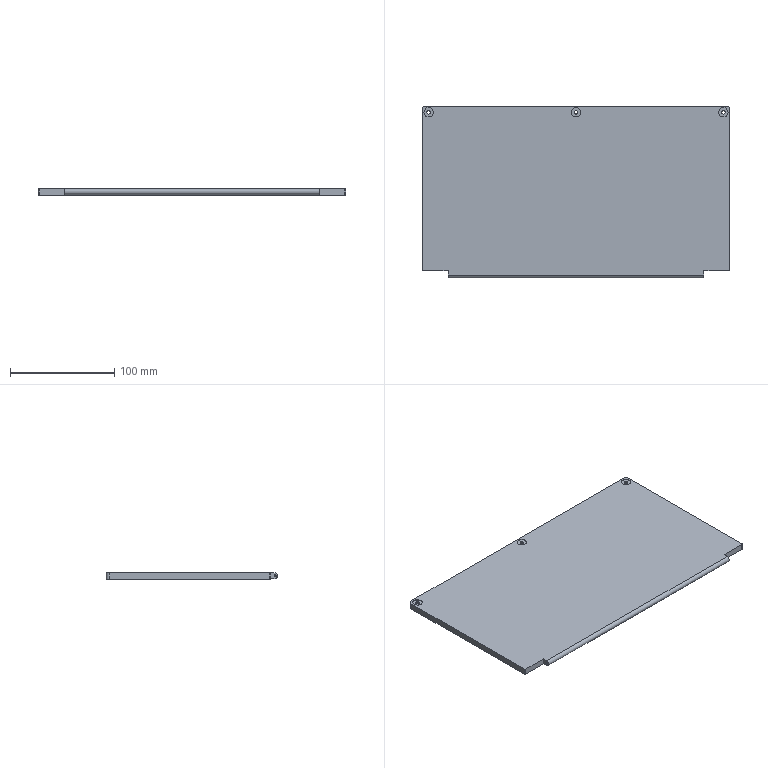NC program | Mastercam | posted with a generic post
Lines 1 to 867 of 5159:
%
O0000()
(MATERIAL - ALUMINUM MM - 2024)
( T9 | 10 FEM | H9 | XY STOCK TO LEAVE - 5. | Z STOCK TO LEAVE - .05 )
( T10 | 10 FEM | H10 | XY STOCK TO LEAVE - 0. | Z STOCK TO LEAVE - .05 )
( T1 | 4 BNOS | H1 )
( T6 | 6 FEM | H6 | XY STOCK TO LEAVE - -.01 | Z STOCK TO LEAVE - 0. )
( T5 | 4 CHM | H5 )
( T3 | 3 FEM | H3 | XY STOCK TO LEAVE - -.01 | Z STOCK TO LEAVE - 0. )
( T8 | 8 FEM | H8 | XY STOCK TO LEAVE - .1 | Z STOCK TO LEAVE - .1 )
N100 G21
N110 G0 G17 G40 G49 G80 G90
N120 T9 M6
N130 G0 G90 G54 X-132.7 Y-102.5 A0. S7000 M3
N140 G43 H9 Z50. M8
N150 Z1.
N160 G1 Z-.496 F600.
N170 Y-92.5 F3000.
N180 Y-85.5
N190 X-146.5
N200 X-156.5
N210 Z-.992 F600.
N220 X-146.5 F3000.
N230 X-132.7
N240 Y-92.5
N250 Y-102.5
N260 Z-1.488 F600.
N270 Y-92.5 F3000.
N280 Y-85.5
N290 X-146.5
N300 X-156.5
N310 Z-1.983 F600.
N320 X-146.5 F3000.
N330 X-132.7
N340 Y-92.5
N350 Y-102.5
N360 Z-2.479 F600.
N370 Y-92.5 F3000.
N380 Y-85.5
N390 X-146.5
N400 X-156.5
N410 Z-2.975 F600.
N420 X-146.5 F3000.
N430 X-132.7
N440 Y-92.5
N450 Y-102.5
N460 Z-3.471 F600.
N470 Y-92.5 F3000.
N480 Y-85.5
N490 X-146.5
N500 X-156.5
N510 Z-3.967 F600.
N520 X-146.5 F3000.
N530 X-132.7
N540 Y-92.5
N550 Y-102.5
N560 Z-4.463 F600.
N570 Y-92.5 F3000.
N580 Y-85.5
N590 X-146.5
N600 X-156.5
N610 Z-4.958 F600.
N620 X-146.5 F3000.
N630 X-132.7
N640 Y-92.5
N650 Y-102.5
N660 Z-5.454 F600.
N670 Y-92.5 F3000.
N680 Y-85.5
N690 X-146.5
N700 X-156.5
N710 Z-5.95 F600.
N720 X-146.5 F3000.
N730 X-132.7
N740 Y-92.5
N750 Y-102.5
N760 G0 Z50.
N770 X156.5 Y-85.5
N780 Z1.
N790 G1 Z-.496 F600.
N800 X146.5 F3000.
N810 X132.7
N820 Y-92.5
N830 Y-102.5
N840 Z-.992 F600.
N850 Y-92.5 F3000.
N860 Y-85.5
N870 X146.5
N880 X156.5
N890 Z-1.488 F600.
N900 X146.5 F3000.
N910 X132.7
N920 Y-92.5
N930 Y-102.5
N940 Z-1.983 F600.
N950 Y-92.5 F3000.
N960 Y-85.5
N970 X146.5
N980 X156.5
N990 Z-2.479 F600.
N1000 X146.5 F3000.
N1010 X132.7
N1020 Y-92.5
N1030 Y-102.5
N1040 Z-2.975 F600.
N1050 Y-92.5 F3000.
N1060 Y-85.5
N1070 X146.5
N1080 X156.5
N1090 Z-3.471 F600.
N1100 X146.5 F3000.
N1110 X132.7
N1120 Y-92.5
N1130 Y-102.5
N1140 Z-3.967 F600.
N1150 Y-92.5 F3000.
N1160 Y-85.5
N1170 X146.5
N1180 X156.5
N1190 Z-4.463 F600.
N1200 X146.5 F3000.
N1210 X132.7
N1220 Y-92.5
N1230 Y-102.5
N1240 Z-4.958 F600.
N1250 Y-92.5 F3000.
N1260 Y-85.5
N1270 X146.5
N1280 X156.5
N1290 Z-5.454 F600.
N1300 X146.5 F3000.
N1310 X132.7
N1320 Y-92.5
N1330 Y-102.5
N1340 Z-5.95 F600.
N1350 Y-92.5 F3000.
N1360 Y-85.5
N1370 X146.5
N1380 X156.5
N1390 G0 Z50.
N1400 X-145.5 Y89.65
N1410 Z1.
N1420 G1 Z0. F600.
N1430 Y88.65 F3000.
N1440 G3 X-144.5 Y87.65 I1. J0.
N1450 G1 X144.5 Z-.153
N1460 G2 X152.65 Y79.5 Z-.16 I0. J-8.15
N1470 G1 Y-74.5 Z-.241
N1480 G2 X146.5 Y-80.65 Z-.246 I-6.15 J0.
N1490 G1 X128.2 Z-.256
N1500 G3 X127.85 Y-81. I0. J-.35
N1510 G1 Y-82.5 Z-.257
N1520 G2 X122.7 Y-87.65 Z-.262 I-5.15 J0.
N1530 G1 X-122.7 Z-.391
N1540 G2 X-127.85 Y-82.5 Z-.396 I0. J5.15
N1550 G1 Y-81. Z-.397
N1560 G3 X-128.2 Y-80.65 I-.35 J0.
N1570 G1 X-146.5 Z-.407
N1580 G2 X-152.65 Y-74.5 Z-.412 I0. J6.15
N1590 G1 Y79.5 Z-.493
N1600 G2 X-144.5 Y87.65 Z-.5 I8.15 J0.
N1610 G1 X144.5 Z-.653
N1620 G2 X152.65 Y79.5 Z-.66 I0. J-8.15
N1630 G1 Y-74.5 Z-.741
N1640 G2 X146.5 Y-80.65 Z-.746 I-6.15 J0.
N1650 G1 X128.2 Z-.756
N1660 G3 X127.85 Y-81. I0. J-.35
N1670 G1 Y-82.5 Z-.757
N1680 G2 X122.7 Y-87.65 Z-.762 I-5.15 J0.
N1690 G1 X-122.7 Z-.891
N1700 G2 X-127.85 Y-82.5 Z-.896 I0. J5.15
N1710 G1 Y-81. Z-.897
N1720 G3 X-128.2 Y-80.65 I-.35 J0.
N1730 G1 X-146.5 Z-.907
N1740 G2 X-152.65 Y-74.5 Z-.912 I0. J6.15
N1750 G1 Y79.5 Z-.993
N1760 G2 X-144.5 Y87.65 Z-1. I8.15 J0.
N1770 G1 X144.5 Z-1.153
N1780 G2 X152.65 Y79.5 Z-1.16 I0. J-8.15
N1790 G1 Y-74.5 Z-1.241
N1800 G2 X146.5 Y-80.65 Z-1.246 I-6.15 J0.
N1810 G1 X128.2 Z-1.256
N1820 G3 X127.85 Y-81. I0. J-.35
N1830 G1 Y-82.5 Z-1.257
N1840 G2 X122.7 Y-87.65 Z-1.262 I-5.15 J0.
N1850 G1 X-122.7 Z-1.391
N1860 G2 X-127.85 Y-82.5 Z-1.396 I0. J5.15
N1870 G1 Y-81. Z-1.397
N1880 G3 X-128.2 Y-80.65 I-.35 J0.
N1890 G1 X-146.5 Z-1.407
N1900 G2 X-152.65 Y-74.5 Z-1.412 I0. J6.15
N1910 G1 Y79.5 Z-1.493
N1920 G2 X-144.5 Y87.65 Z-1.5 I8.15 J0.
N1930 G1 X144.5 Z-1.653
N1940 G2 X152.65 Y79.5 Z-1.66 I0. J-8.15
N1950 G1 Y-74.5 Z-1.741
N1960 G2 X146.5 Y-80.65 Z-1.746 I-6.15 J0.
N1970 G1 X128.2 Z-1.756
N1980 G3 X127.85 Y-81. I0. J-.35
N1990 G1 Y-82.5 Z-1.757
N2000 G2 X122.7 Y-87.65 Z-1.762 I-5.15 J0.
N2010 G1 X-122.7 Z-1.891
N2020 G2 X-127.85 Y-82.5 Z-1.896 I0. J5.15
N2030 G1 Y-81. Z-1.897
N2040 G3 X-128.2 Y-80.65 I-.35 J0.
N2050 G1 X-146.5 Z-1.907
N2060 G2 X-152.65 Y-74.5 Z-1.912 I0. J6.15
N2070 G1 Y79.5 Z-1.993
N2080 G2 X-144.5 Y87.65 Z-2. I8.15 J0.
N2090 G1 X144.5 Z-2.153
N2100 G2 X152.65 Y79.5 Z-2.16 I0. J-8.15
N2110 G1 Y-74.5 Z-2.241
N2120 G2 X146.5 Y-80.65 Z-2.246 I-6.15 J0.
N2130 G1 X128.2 Z-2.256
N2140 G3 X127.85 Y-81. I0. J-.35
N2150 G1 Y-82.5 Z-2.257
N2160 G2 X122.7 Y-87.65 Z-2.262 I-5.15 J0.
N2170 G1 X-122.7 Z-2.391
N2180 G2 X-127.85 Y-82.5 Z-2.396 I0. J5.15
N2190 G1 Y-81. Z-2.397
N2200 G3 X-128.2 Y-80.65 I-.35 J0.
N2210 G1 X-146.5 Z-2.407
N2220 G2 X-152.65 Y-74.5 Z-2.412 I0. J6.15
N2230 G1 Y79.5 Z-2.493
N2240 G2 X-144.5 Y87.65 Z-2.5 I8.15 J0.
N2250 G1 X144.5 Z-2.653
N2260 G2 X152.65 Y79.5 Z-2.66 I0. J-8.15
N2270 G1 Y-74.5 Z-2.741
N2280 G2 X146.5 Y-80.65 Z-2.746 I-6.15 J0.
N2290 G1 X128.2 Z-2.756
N2300 G3 X127.85 Y-81. I0. J-.35
N2310 G1 Y-82.5 Z-2.757
N2320 G2 X122.7 Y-87.65 Z-2.762 I-5.15 J0.
N2330 G1 X-122.7 Z-2.891
N2340 G2 X-127.85 Y-82.5 Z-2.896 I0. J5.15
N2350 G1 Y-81. Z-2.897
N2360 G3 X-128.2 Y-80.65 I-.35 J0.
N2370 G1 X-146.5 Z-2.907
N2380 G2 X-152.65 Y-74.5 Z-2.912 I0. J6.15
N2390 G1 Y79.5 Z-2.993
N2400 G2 X-144.5 Y87.65 Z-3. I8.15 J0.
N2410 G1 X144.5 Z-3.153
N2420 G2 X152.65 Y79.5 Z-3.16 I0. J-8.15
N2430 G1 Y-74.5 Z-3.241
N2440 G2 X146.5 Y-80.65 Z-3.246 I-6.15 J0.
N2450 G1 X128.2 Z-3.256
N2460 G3 X127.85 Y-81. I0. J-.35
N2470 G1 Y-82.5 Z-3.257
N2480 G2 X122.7 Y-87.65 Z-3.262 I-5.15 J0.
N2490 G1 X-122.7 Z-3.391
N2500 G2 X-127.85 Y-82.5 Z-3.396 I0. J5.15
N2510 G1 Y-81. Z-3.397
N2520 G3 X-128.2 Y-80.65 I-.35 J0.
N2530 G1 X-146.5 Z-3.407
N2540 G2 X-152.65 Y-74.5 Z-3.412 I0. J6.15
N2550 G1 Y79.5 Z-3.493
N2560 G2 X-144.5 Y87.65 Z-3.5 I8.15 J0.
N2570 G1 X144.5 Z-3.653
N2580 G2 X152.65 Y79.5 Z-3.66 I0. J-8.15
N2590 G1 Y-74.5 Z-3.741
N2600 G2 X146.5 Y-80.65 Z-3.746 I-6.15 J0.
N2610 G1 X128.2 Z-3.756
N2620 G3 X127.85 Y-81. I0. J-.35
N2630 G1 Y-82.5 Z-3.757
N2640 G2 X122.7 Y-87.65 Z-3.762 I-5.15 J0.
N2650 G1 X-122.7 Z-3.891
N2660 G2 X-127.85 Y-82.5 Z-3.896 I0. J5.15
N2670 G1 Y-81. Z-3.897
N2680 G3 X-128.2 Y-80.65 I-.35 J0.
N2690 G1 X-146.5 Z-3.907
N2700 G2 X-152.65 Y-74.5 Z-3.912 I0. J6.15
N2710 G1 Y79.5 Z-3.993
N2720 G2 X-144.5 Y87.65 Z-4. I8.15 J0.
N2730 G1 X144.5 Z-4.153
N2740 G2 X152.65 Y79.5 Z-4.16 I0. J-8.15
N2750 G1 Y-74.5 Z-4.241
N2760 G2 X146.5 Y-80.65 Z-4.246 I-6.15 J0.
N2770 G1 X128.2 Z-4.256
N2780 G3 X127.85 Y-81. I0. J-.35
N2790 G1 Y-82.5 Z-4.257
N2800 G2 X122.7 Y-87.65 Z-4.262 I-5.15 J0.
N2810 G1 X-122.7 Z-4.391
N2820 G2 X-127.85 Y-82.5 Z-4.396 I0. J5.15
N2830 G1 Y-81. Z-4.397
N2840 G3 X-128.2 Y-80.65 I-.35 J0.
N2850 G1 X-146.5 Z-4.407
N2860 G2 X-152.65 Y-74.5 Z-4.412 I0. J6.15
N2870 G1 Y79.5 Z-4.493
N2880 G2 X-144.5 Y87.65 Z-4.5 I8.15 J0.
N2890 G1 X144.5 Z-4.653
N2900 G2 X152.65 Y79.5 Z-4.66 I0. J-8.15
N2910 G1 Y-74.5 Z-4.741
N2920 G2 X146.5 Y-80.65 Z-4.746 I-6.15 J0.
N2930 G1 X128.2 Z-4.756
N2940 G3 X127.85 Y-81. I0. J-.35
N2950 G1 Y-82.5 Z-4.757
N2960 G2 X122.7 Y-87.65 Z-4.762 I-5.15 J0.
N2970 G1 X-122.7 Z-4.891
N2980 G2 X-127.85 Y-82.5 Z-4.896 I0. J5.15
N2990 G1 Y-81. Z-4.897
N3000 G3 X-128.2 Y-80.65 I-.35 J0.
N3010 G1 X-146.5 Z-4.907
N3020 G2 X-152.65 Y-74.5 Z-4.912 I0. J6.15
N3030 G1 Y79.5 Z-4.993
N3040 G2 X-144.5 Y87.65 Z-5. I8.15 J0.
N3050 G1 X144.5 Z-5.153
N3060 G2 X152.65 Y79.5 Z-5.16 I0. J-8.15
N3070 G1 Y-74.5 Z-5.241
N3080 G2 X146.5 Y-80.65 Z-5.246 I-6.15 J0.
N3090 G1 X128.2 Z-5.256
N3100 G3 X127.85 Y-81. I0. J-.35
N3110 G1 Y-82.5 Z-5.257
N3120 G2 X122.7 Y-87.65 Z-5.262 I-5.15 J0.
N3130 G1 X-122.7 Z-5.391
N3140 G2 X-127.85 Y-82.5 Z-5.396 I0. J5.15
N3150 G1 Y-81. Z-5.397
N3160 G3 X-128.2 Y-80.65 I-.35 J0.
N3170 G1 X-146.5 Z-5.407
N3180 G2 X-152.65 Y-74.5 Z-5.412 I0. J6.15
N3190 G1 Y79.5 Z-5.493
N3200 G2 X-144.5 Y87.65 Z-5.5 I8.15 J0.
N3210 G1 X144.5 Z-5.653
N3220 G2 X152.65 Y79.5 Z-5.66 I0. J-8.15
N3230 G1 Y-74.5 Z-5.741
N3240 G2 X146.5 Y-80.65 Z-5.746 I-6.15 J0.
N3250 G1 X128.2 Z-5.756
N3260 G3 X127.85 Y-81. I0. J-.35
N3270 G1 Y-82.5 Z-5.757
N3280 G2 X122.7 Y-87.65 Z-5.762 I-5.15 J0.
N3290 G1 X-122.7 Z-5.891
N3300 G2 X-127.85 Y-82.5 Z-5.896 I0. J5.15
N3310 G1 Y-81. Z-5.897
N3320 G3 X-128.2 Y-80.65 I-.35 J0.
N3330 G1 X-146.5 Z-5.907
N3340 G2 X-152.65 Y-74.5 Z-5.912 I0. J6.15
N3350 G1 Y-2.118 Z-5.95
N3360 Y79.5
N3370 G2 X-144.5 Y87.65 I8.15 J0.
N3380 G1 X144.5
N3390 G2 X152.65 Y79.5 I0. J-8.15
N3400 G1 Y-74.5
N3410 G2 X146.5 Y-80.65 I-6.15 J0.
N3420 G1 X128.2
N3430 G3 X127.85 Y-81. I0. J-.35
N3440 G1 Y-82.5
N3450 G2 X122.7 Y-87.65 I-5.15 J0.
N3460 G1 X-122.7
N3470 G2 X-127.85 Y-82.5 I0. J5.15
N3480 G1 Y-81.
N3490 G3 X-128.2 Y-80.65 I-.35 J0.
N3500 G1 X-146.5
N3510 G2 X-152.65 Y-74.5 I0. J6.15
N3520 G1 Y-2.118
N3530 G3 X-153.65 Y-1.118 I-1. J0.
N3540 G1 X-154.65
N3550 G0 Z50.
N3560 M5
N3570 G91 G28 Z0. M9
N3580 A0.
N3590 M01
N3600 T10 M6
N3610 G0 G90 G17 G54 X-145.5 Y89.5 A0. S7000 M3
N3620 G43 H10 Z50. M8
N3630 Z1.
N3640 G1 Z-5.95 F600.
N3650 Y88.5 F1000.
N3660 G3 X-144.5 Y87.5 I1. J0.
N3670 G1 X144.5
N3680 G2 X152.5 Y79.5 I0. J-8.
N3690 G1 Y-74.5
N3700 G2 X146.5 Y-80.5 I-6. J0.
N3710 G1 X128.2
N3720 G3 X127.7 Y-81. I0. J-.5
N3730 G1 Y-82.5
N3740 G2 X122.7 Y-87.5 I-5. J0.
N3750 G1 X-122.7
N3760 G2 X-127.7 Y-82.5 I0. J5.
N3770 G1 Y-81.
N3780 G3 X-128.2 Y-80.5 I-.5 J0.
N3790 G1 X-146.5
N3800 G2 X-152.5 Y-74.5 I0. J6.
N3810 G1 Y79.5
N3820 G2 X-144.5 Y87.5 I8. J0.
N3830 G3 X-143.5 Y88.5 I0. J1.
N3840 G1 Y89.5
N3850 G0 Z50.
N3860 M5
N3870 G91 G28 Z0. M9
N3880 A0.
N3890 M01
N3900 T1 M6
N3910 G0 G90 G17 G54 X132.7 Y-84.49 A0. S10000 M3
N3920 G43 H1 Z50. M8
N3930 Z.929
N3940 G1 Z-3.693 F600.
N3950 X122.7 F3000.
N3960 Z-4.071 F600.
N3970 X-122.7 F3000.
N3980 Z-3.693
N3990 X-132.7
N4000 Z-3.936
N4010 Y-84.498
N4020 X-122.7
N4030 X122.7
N4040 X132.7
N4050 Z-3.8
N4060 Y-84.5
N4070 X122.7
N4080 X-122.7
N4090 X-132.7
N4100 Z-3.664
N4110 Y-84.498
N4120 X-122.7
N4130 X122.7
N4140 X132.7
N4150 Z-3.529
N4160 Y-84.49
N4170 X122.7
N4180 X-122.7
N4190 X-132.7
N4200 Z-3.394
N4210 Y-84.478
N4220 X-122.7
N4230 X122.7
N4240 X132.7
N4250 Z-3.26
N4260 Y-84.461
N4270 X122.7
N4280 X-122.7
N4290 X-132.7
N4300 Z-3.127
N4310 Y-84.44
N4320 X-122.7
N4330 X122.7
N4340 X132.7
N4350 Z-2.996
N4360 Y-84.414
N4370 X122.7
N4380 X-122.7
N4390 X-132.7
N4400 Z-2.865
N4410 Y-84.383
N4420 X-122.7
N4430 X122.7
N4440 X132.7
N4450 Z-2.737
N4460 Y-84.348
N4470 X122.7
N4480 X-122.7
N4490 X-132.7
N4500 Z-2.61
N4510 Y-84.309
N4520 X-122.7
N4530 X122.7
N4540 X132.7
N4550 Z-2.486
N4560 Y-84.265
N4570 X122.7
N4580 X-122.7
N4590 X-132.7
N4600 Z-2.364
N4610 Y-84.218
N4620 X-122.7
N4630 X122.7
N4640 X132.7
N4650 Z-2.244
N4660 Y-84.167
N4670 X122.7
N4680 X-122.7
N4690 X-132.7
N4700 Z-2.127
N4710 Y-84.112
N4720 X-122.7
N4730 X122.7
N4740 X132.7
N4750 Z-2.013
N4760 Y-84.054
N4770 X122.7
N4780 X-122.7
N4790 X-132.7
N4800 Z-1.902
N4810 Y-83.992
N4820 X-122.7
N4830 X122.7
N4840 X132.7
N4850 Z-1.794
N4860 Y-83.927
N4870 X122.7
N4880 X-122.7
N4890 X-132.7
N4900 Z-1.689
N4910 Y-83.86
N4920 X-122.7
N4930 X122.7
N4940 X132.7
N4950 Z-1.587
N4960 Y-83.789
N4970 X122.7
N4980 X-122.7
N4990 X-132.7
N5000 Z-1.489
N5010 Y-83.716
N5020 X-122.7
N5030 X122.7
N5040 X132.7
N5050 Z-1.394
N5060 Y-83.641
N5070 X122.7
N5080 X-122.7
N5090 X-132.7
N5100 Z-1.303
N5110 Y-83.564
N5120 X-122.7
N5130 X122.7
N5140 X132.7
N5150 Z-1.215
N5160 Y-83.485
N5170 X122.7
N5180 X-122.7
N5190 X-132.7
N5200 Z-1.13
N5210 Y-83.404
N5220 X-122.7
N5230 X122.7
N5240 X132.7
N5250 Z-1.05
N5260 Y-83.322
N5270 X122.7
N5280 X-122.7
N5290 X-132.7
N5300 Z-.972
N5310 Y-83.239
N5320 X-122.7
N5330 X122.7
N5340 X132.7
N5350 Z-.899
N5360 Y-83.154
N5370 X122.7
N5380 X-122.7
N5390 X-132.7
N5400 Z-.828
N5410 Y-83.068
N5420 X-122.7
N5430 X122.7
N5440 X132.7
N5450 Z-.761
N5460 Y-82.982
N5470 X122.7
N5480 X-122.7
N5490 X-132.7
N5500 Z-.681
N5510 Y-82.871
N5520 X-122.7
N5530 X122.7
N5540 X132.7
N5550 Z-.606
N5560 Y-82.759
N5570 X122.7
N5580 X-122.7
N5590 X-132.7
N5600 Z-.537
N5610 Y-82.647
N5620 X-122.7
N5630 X122.7
N5640 X132.7
N5650 Z-.472
N5660 Y-82.535
N5670 X122.7
N5680 X-122.7
N5690 X-132.7
N5700 Z-.413
N5710 Y-82.423
N5720 X-122.7
N5730 X122.7
N5740 X132.7
N5750 Z-.358
N5760 Y-82.311
N5770 X122.7
N5780 X-122.7
N5790 X-132.7
N5800 Z-.309
N5810 Y-82.2
N5820 X-122.7
N5830 X122.7
N5840 X132.7
N5850 Z-.263
N5860 Y-82.09
N5870 X122.7
N5880 X-122.7
N5890 X-132.7
N5900 Z-.222
N5910 Y-81.98
N5920 X-122.7
N5930 X122.7
N5940 X132.7
N5950 Z-.185
N5960 Y-81.872
N5970 X122.7
N5980 X-122.7
N5990 X-132.7
N6000 Z-.152
N6010 Y-81.765
N6020 X-122.7
N6030 X122.7
N6040 X132.7
N6050 Z-.123
N6060 Y-81.66
N6070 X122.7
N6080 X-122.7
N6090 X-132.7
N6100 Z-.098
N6110 Y-81.556
N6120 X-122.7
N6130 X122.7
N6140 X132.7
N6150 Z-.075
N6160 Y-81.453
N6170 X122.7
N6180 X-122.7
N6190 X-132.7
N6200 Z-.056
N6210 Y-81.353
N6220 X-122.7
N6230 X122.7
N6240 X132.7
N6250 Z-.041
N6260 Y-81.254
N6270 X122.7
N6280 X-122.7
N6290 X-132.7
N6300 Z-.028
N6310 Y-81.157
N6320 X-122.7
N6330 X122.7
N6340 X132.7
N6350 Z-.017
N6360 Y-81.061
N6370 X122.7
N6380 X-122.7
N6390 X-132.7
N6400 Z-.009
N6410 Y-80.968
N6420 X-122.7
N6430 X122.7
N6440 X132.7
N6450 Z-.004
N6460 Y-80.877
N6470 X122.7
N6480 X-122.7
N6490 X-132.7
N6500 Z-.001
N6510 Y-80.787
N6520 X-122.7
N6530 X122.7
N6540 X132.7
N6550 Z0.
N6560 Y-80.7
N6570 X122.7
N6580 X-122.7
N6590 X-132.7
N6600 G0 Z5.
N6610 Z50.
N6620 M5
N6630 G91 G28 Z0. M9
N6640 A0.
N6650 M01
N6660 T6 M6
N6670 G0 G90 G17 G54 X0. Y76.5 A0. S7000 M3
N6680 G43 H6 Z50. M8
N6690 Z1.
N6700 G1 Z0. F600.
N6710 X-.329 Y75.559 F3000.
N6720 G3 X.306 Y75.16 I.635 J.306
N6730 X.612 Y75.23 I0. J.705
N6740 X1.41 Y76.5 Z-.062 I-.612 J1.27
N6750 X0. Y77.91 Z-.15 I-1.41 J0.
N6760 X-1.41 Y76.5 Z-.237 I0. J-1.41
N6770 X0. Y75.09 Z-.325 I1.41 J0.
N6780 X.612 Y75.23 Z-.35 I0. J1.41
N6790 X1.41 Y76.5 Z-.412 I-.612 J1.27
N6800 X0. Y77.91 Z-.5 I-1.41 J0.
N6810 X-1.41 Y76.5 I0. J-1.41 F1500.
N6820 X0. Y75.09 I1.41 J0.
N6830 X1.41 Y76.5 I0. J1.41
N6840 X0. Y77.91 I-1.41 J0.
N6850 X-.49 Y77.822 I0. J-1.41
N6860 X-.95 Y77.161 I.245 J-.661
N6870 X-.906 Y76.916 I.705 J0.
N6880 G1 X0. Y76.5
N6890 G0 Z0.
N6900 G1 X.755 Y77.255 F750.
N6910 G3 X0. Y78.01 I-.755 J0.
N6920 X-1.51 Y76.5 I0. J-1.51
N6930 X0. Y74.99 I1.51 J0.
N6940 X1.51 Y76.5 I0. J1.51
N6950 X0. Y78.01 I-1.51 J0.
N6960 X-.491 Y77.928 I0. J-1.51
N6970 X-1.482 Y76.789 Z-.5 I.491 J-1.428
N6980 X-1.51 Y76.5 I1.482 J-.289
N6990 X0. Y74.99 I1.51 J0.
N7000 X1.51 Y76.5 I0. J1.51
N7010 X0. Y78.01 I-1.51 J0.
N7020 X-1.482 Y76.789 I0. J-1.51
N7030 X-1.51 Y76.5 I1.482 J-.289
N7040 X-1.496 Y76.291 I1.51 J0.
N7050 X-.748 Y75.641 I.748 J.105
N7060 X-.643 Y75.648 I0. J.755
N7070 G1 X0. Y76.5
N7080 G0 Z50.
N7090 X-141.5
N7100 Z1.
N7110 G1 Z0. F600.
N7120 X-141.829 Y75.559 F3000.
N7130 G3 X-141.194 Y75.16 I.635 J.306
N7140 X-140.888 Y75.23 I0. J.705
N7150 X-140.09 Y76.5 Z-.062 I-.612 J1.27
N7160 X-141.5 Y77.91 Z-.15 I-1.41 J0.
N7170 X-142.91 Y76.5 Z-.237 I0. J-1.41
N7180 X-141.5 Y75.09 Z-.325 I1.41 J0.
N7190 X-140.888 Y75.23 Z-.35 I0. J1.41
N7200 X-140.09 Y76.5 Z-.412 I-.612 J1.27
N7210 X-141.5 Y77.91 Z-.5 I-1.41 J0.
N7220 X-142.91 Y76.5 I0. J-1.41 F1500.
N7230 X-141.5 Y75.09 I1.41 J0.
N7240 X-140.09 Y76.5 I0. J1.41
N7250 X-141.5 Y77.91 I-1.41 J0.
N7260 X-141.99 Y77.822 I0. J-1.41
N7270 X-142.45 Y77.161 I.245 J-.661
N7280 X-142.406 Y76.916 I.705 J0.
N7290 G1 X-141.5 Y76.5
N7300 G0 Z0.
N7310 G1 X-140.745 Y77.255 F750.
N7320 G3 X-141.5 Y78.01 I-.755 J0.
N7330 X-143.01 Y76.5 I0. J-1.51
N7340 X-141.5 Y74.99 I1.51 J0.
N7350 X-139.99 Y76.5 I0. J1.51
N7360 X-141.5 Y78.01 I-1.51 J0.
N7370 X-141.991 Y77.928 I0. J-1.51
N7380 X-142.982 Y76.789 Z-.5 I.491 J-1.428
N7390 X-143.01 Y76.5 I1.482 J-.289
N7400 X-141.5 Y74.99 I1.51 J0.
N7410 X-139.99 Y76.5 I0. J1.51
N7420 X-141.5 Y78.01 I-1.51 J0.
N7430 X-142.982 Y76.789 I0. J-1.51
N7440 X-143.01 Y76.5 I1.482 J-.289
N7450 X-142.996 Y76.291 I1.51 J0.
N7460 X-142.248 Y75.641 I.748 J.105
N7470 X-142.143 Y75.648 I0. J.755
N7480 G1 X-141.5 Y76.5
N7490 G0 Z50.
N7500 X141.5
N7510 Z1.
N7520 G1 Z0. F600.
N7530 X141.171 Y75.559 F3000.
N7540 G3 X141.806 Y75.16 I.635 J.306
N7550 X142.112 Y75.23 I0. J.705
N7560 X142.91 Y76.5 Z-.062 I-.612 J1.27
N7570 X141.5 Y77.91 Z-.15 I-1.41 J0.
N7580 X140.09 Y76.5 Z-.237 I0. J-1.41
N7590 X141.5 Y75.09 Z-.325 I1.41 J0.
N7600 X142.112 Y75.23 Z-.35 I0. J1.41
N7610 X142.91 Y76.5 Z-.412 I-.612 J1.27
N7620 X141.5 Y77.91 Z-.5 I-1.41 J0.
N7630 X140.09 Y76.5 I0. J-1.41 F1500.
N7640 X141.5 Y75.09 I1.41 J0.
N7650 X142.91 Y76.5 I0. J1.41
N7660 X141.5 Y77.91 I-1.41 J0.
N7670 X141.01 Y77.822 I0. J-1.41
N7680 X140.55 Y77.161 I.245 J-.661
N7690 X140.594 Y76.916 I.705 J0.
N7700 G1 X141.5 Y76.5
N7710 G0 Z0.
N7720 G1 X142.255 Y77.255 F750.
N7730 G3 X141.5 Y78.01 I-.755 J0.
N7740 X139.99 Y76.5 I0. J-1.51
N7750 X141.5 Y74.99 I1.51 J0.
N7760 X143.01 Y76.5 I0. J1.51
N7770 X141.5 Y78.01 I-1.51 J0.
N7780 X141.009 Y77.928 I0. J-1.51
N7790 X140.018 Y76.789 Z-.5 I.491 J-1.428
N7800 X139.99 Y76.5 I1.482 J-.289
N7810 X141.5 Y74.99 I1.51 J0.
N7820 X143.01 Y76.5 I0. J1.51
N7830 X141.5 Y78.01 I-1.51 J0.
N7840 X140.018 Y76.789 I0. J-1.51
N7850 X139.99 Y76.5 I1.482 J-.289
N7860 X140.004 Y76.291 I1.51 J0.
N7870 X140.752 Y75.641 I.748 J.105
N7880 X140.857 Y75.648 I0. J.755
N7890 G1 X141.5 Y76.5
N7900 G0 Z50.
N7910 M5
N7920 G91 G28 Z0. M9
N7930 A0.
N7940 M01
N7950 T5 M6
N7960 G0 G90 G17 G54 X0. Y76.5 A0. S3000 M3
N7970 G43 H5 Z49.5 M8
N7980 G98 G81 Z-1.2 R.5 F300.
N7990 X-141.5
N8000 X141.5
N8010 G80
N8020 S7000 M3
N8030 G0 X-138.15 Y76.1 Z50.
N8040 Z1.
N8050 G1 Z-.4 F600.
N8060 X-137.75 F1000.
N8070 G3 X-137.35 Y76.5 I0. J.4
N8080 X-141.5 Y80.65 I-4.15 J0.
N8090 X-145.65 Y76.5 I0. J-4.15
N8100 X-141.5 Y72.35 I4.15 J0.
N8110 X-137.35 Y76.5 I0. J4.15
N8120 X-137.75 Y76.9 I-.4 J0.
N8130 G1 X-138.15
N8140 G0 Z50.
N8150 X3.35 Y76.1
N8160 Z1.
N8170 G1 Z-.4 F600.
N8180 X3.75 F1000.
N8190 G3 X4.15 Y76.5 I0. J.4
N8200 X0. Y80.65 I-4.15 J0.
N8210 X-4.15 Y76.5 I0. J-4.15
N8220 X0. Y72.35 I4.15 J0.
N8230 X4.15 Y76.5 I0. J4.15
N8240 X3.75 Y76.9 I-.4 J0.
N8250 G1 X3.35
N8260 G0 Z50.
N8270 X144.85 Y76.1
N8280 Z1.
N8290 G1 Z-.4 F600.
N8300 X145.25 F1000.
N8310 G3 X145.65 Y76.5 I0. J.4
N8320 X141.5 Y80.65 I-4.15 J0.
N8330 X137.35 Y76.5 I0. J-4.15
N8340 X141.5 Y72.35 I4.15 J0.
N8350 X145.65 Y76.5 I0. J4.15
N8360 X145.25 Y76.9 I-.4 J0.
N8370 G1 X144.85
N8380 G0 Z50.
N8390 X-148.95 Y-74.9
N8400 Z1.
N8410 G1 Z-.8 F600.
N8420 X-148.55 F1000.
N8430 G3 X-148.15 Y-74.5 I0. J.4
N8440 G1 Y79.5
N8450 G2 X-144.5 Y83.15 I3.65 J0.
N8460 G1 X144.5
N8470 G2 X148.15 Y79.5 I0. J-3.65
N8480 G1 Y-74.5
N8490 G2 X146.5 Y-76.15 I-1.65 J0.
N8500 G1 X128.2
N8510 G3 X123.35 Y-81. I0. J-4.85
N8520 G1 Y-82.5
N8530 G2 X122.7 Y-83.15 I-.65 J0.
N8540 G1 X-122.7
N8550 G2 X-123.35 Y-82.5 I0. J.65
N8560 G1 Y-81.
N8570 G3 X-128.2 Y-76.15 I-4.85 J0.
N8580 G1 X-146.5
N8590 G2 X-148.15 Y-74.5 I0. J1.65
N8600 G3 X-148.55 Y-74.1 I-.4 J0.
N8610 G1 X-148.95
N8620 G0 Z50.
N8630 M5
N8640 G91 G28 Z0. M9
N8650 A0.
N8660 M01